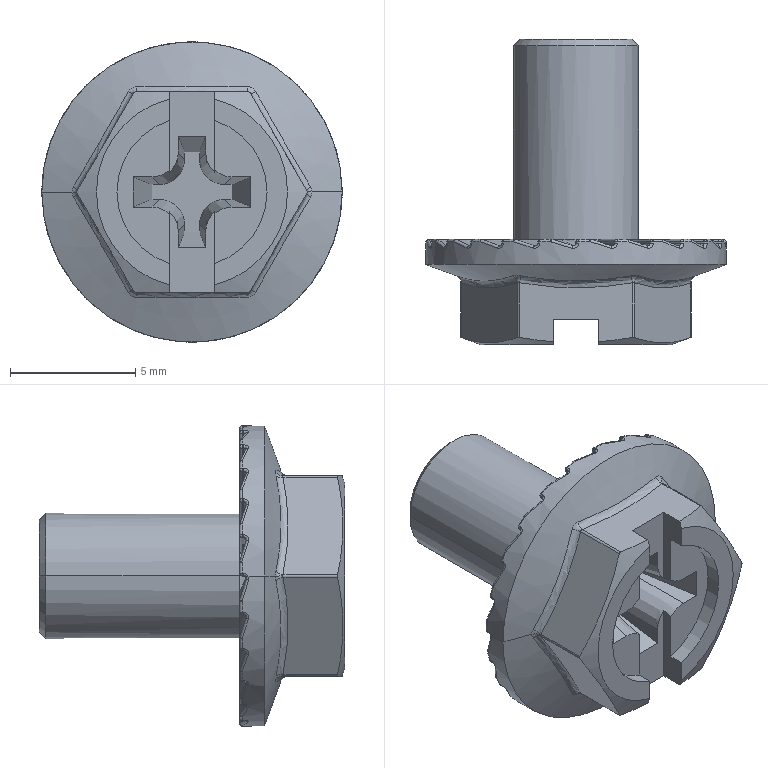Part | STEP file | _X2_751F4E45_X0_MS731-1_X2_8_12 | 1 solid | 357 faces | box 12 x 12.2 x 12 mm | volume 416.607 mm3 | spline 136 | cylinder 84 | plane 55 | sphere 48 | torus 24 | cone 6 | other 4 | commonest cylinder face diameters 0.2 x54 7 x24 5 x2 6 x2 12 x2